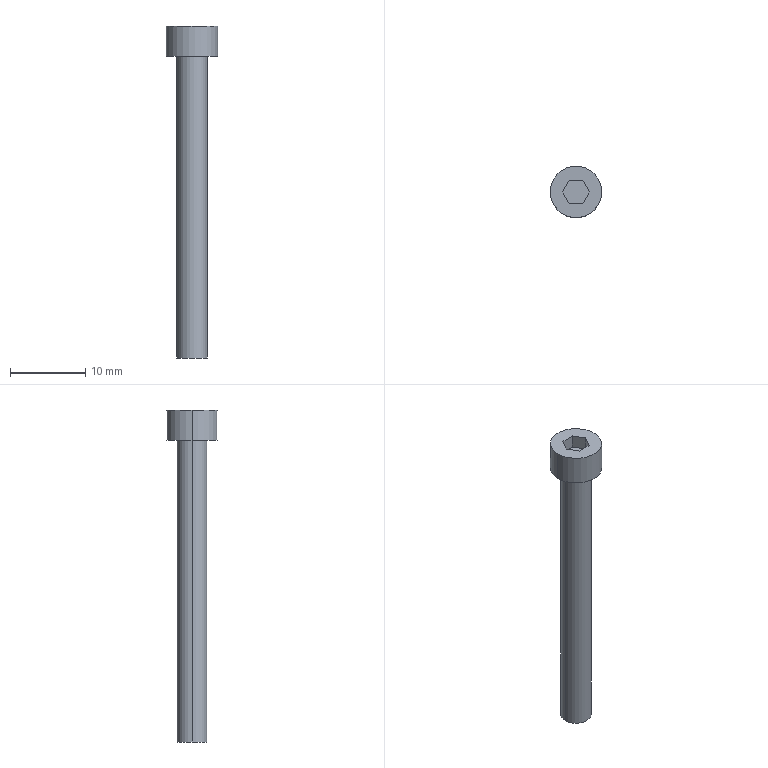Part | SolidWorks | features BaseBody 1 | 1 solid | 14 faces | box 6.8 x 6.8 x 44 mm | volume 632.77 mm3 | plane 10 | cylinder 4 | commonest cylinder face diameters 4 x2 6.8 x2
STEP:
#1=CARTESIAN_POINT('',(2.,0.,-40.));
#2=VERTEX_POINT('',#1);
#3=CARTESIAN_POINT('',(-2.,0.,-40.));
#4=VERTEX_POINT('',#3);
#5=CARTESIAN_POINT('',(0.,0.,-40.));
#6=DIRECTION('',(0.,0.,1.));
#7=DIRECTION('',(1.,0.,0.));
#8=AXIS2_PLACEMENT_3D('',#5,#6,#7);
#9=CIRCLE('',#8,2.);
#10=EDGE_CURVE('',#2,#4,#9,.T.);
#11=ORIENTED_EDGE('',*,*,#10,.T.);
#12=CARTESIAN_POINT('',(-2.,0.,0.));
#13=VERTEX_POINT('',#12);
#14=CARTESIAN_POINT('',(-2.,0.,-40.));
#15=DIRECTION('',(0.,0.,1.));
#16=VECTOR('',#15,1000.);
#17=LINE('',#14,#16);
#18=EDGE_CURVE('',#4,#13,#17,.T.);
#19=ORIENTED_EDGE('',*,*,#18,.T.);
#20=CARTESIAN_POINT('',(2.,0.,0.));
#21=VERTEX_POINT('',#20);
#22=CARTESIAN_POINT('',(0.,0.,0.));
#23=DIRECTION('',(0.,0.,-1.));
#24=DIRECTION('',(1.,0.,0.));
#25=AXIS2_PLACEMENT_3D('',#22,#23,#24);
#26=CIRCLE('',#25,2.);
#27=EDGE_CURVE('',#13,#21,#26,.T.);
#28=ORIENTED_EDGE('',*,*,#27,.T.);
#29=CARTESIAN_POINT('',(2.,0.,-40.));
#30=DIRECTION('',(0.,0.,1.));
#31=VECTOR('',#30,1000.);
#32=LINE('',#29,#31);
#33=EDGE_CURVE('',#2,#21,#32,.T.);
#34=ORIENTED_EDGE('',*,*,#33,.F.);
#35=EDGE_LOOP('',(#11,#19,#28,#34));
#36=FACE_OUTER_BOUND('',#35,.T.);
#37=CARTESIAN_POINT('',(0.,0.,-40.));
#38=DIRECTION('',(0.,0.,1.));
#39=DIRECTION('',(1.,0.,0.));
#40=AXIS2_PLACEMENT_3D('',#37,#38,#39);
#41=CYLINDRICAL_SURFACE('',#40,2.);
#42=ADVANCED_FACE('',(#36),#41,.T.);
#43=CARTESIAN_POINT('',(3.4,0.,0.));
#44=VERTEX_POINT('',#43);
#45=CARTESIAN_POINT('',(-3.4,0.,0.));
#46=VERTEX_POINT('',#45);
#47=CARTESIAN_POINT('',(0.,0.,0.));
#48=DIRECTION('',(0.,0.,1.));
#49=DIRECTION('',(1.,0.,0.));
#50=AXIS2_PLACEMENT_3D('',#47,#48,#49);
#51=CIRCLE('',#50,3.4);
#52=EDGE_CURVE('',#44,#46,#51,.T.);
#53=ORIENTED_EDGE('',*,*,#52,.T.);
#54=CARTESIAN_POINT('',(-3.4,0.,4.));
#55=VERTEX_POINT('',#54);
#56=CARTESIAN_POINT('',(-3.4,0.,0.));
#57=DIRECTION('',(0.,0.,1.));
#58=VECTOR('',#57,1000.);
#59=LINE('',#56,#58);
#60=EDGE_CURVE('',#46,#55,#59,.T.);
#61=ORIENTED_EDGE('',*,*,#60,.T.);
#62=CARTESIAN_POINT('',(3.4,0.,4.));
#63=VERTEX_POINT('',#62);
#64=CARTESIAN_POINT('',(0.,0.,4.));
#65=DIRECTION('',(0.,0.,-1.));
#66=DIRECTION('',(1.,0.,0.));
#67=AXIS2_PLACEMENT_3D('',#64,#65,#66);
#68=CIRCLE('',#67,3.4);
#69=EDGE_CURVE('',#55,#63,#68,.T.);
#70=ORIENTED_EDGE('',*,*,#69,.T.);
#71=CARTESIAN_POINT('',(3.4,0.,0.));
#72=DIRECTION('',(0.,0.,1.));
#73=VECTOR('',#72,1000.);
#74=LINE('',#71,#73);
#75=EDGE_CURVE('',#44,#63,#74,.T.);
#76=ORIENTED_EDGE('',*,*,#75,.F.);
#77=EDGE_LOOP('',(#53,#61,#70,#76));
#78=FACE_OUTER_BOUND('',#77,.T.);
#79=CARTESIAN_POINT('',(0.,0.,0.));
#80=DIRECTION('',(0.,0.,1.));
#81=DIRECTION('',(1.,0.,0.));
#82=AXIS2_PLACEMENT_3D('',#79,#80,#81);
#83=CYLINDRICAL_SURFACE('',#82,3.4);
#84=ADVANCED_FACE('',(#78),#83,.T.);
#85=ORIENTED_EDGE('',*,*,#18,.F.);
#86=CARTESIAN_POINT('',(0.,0.,-40.));
#87=DIRECTION('',(0.,0.,1.));
#88=DIRECTION('',(1.,0.,0.));
#89=AXIS2_PLACEMENT_3D('',#86,#87,#88);
#90=CIRCLE('',#89,2.);
#91=EDGE_CURVE('',#4,#2,#90,.T.);
#92=ORIENTED_EDGE('',*,*,#91,.T.);
#93=ORIENTED_EDGE('',*,*,#33,.T.);
#94=CARTESIAN_POINT('',(0.,0.,0.));
#95=DIRECTION('',(0.,0.,-1.));
#96=DIRECTION('',(1.,0.,0.));
#97=AXIS2_PLACEMENT_3D('',#94,#95,#96);
#98=CIRCLE('',#97,2.);
#99=EDGE_CURVE('',#21,#13,#98,.T.);
#100=ORIENTED_EDGE('',*,*,#99,.T.);
#101=EDGE_LOOP('',(#85,#92,#93,#100));
#102=FACE_OUTER_BOUND('',#101,.T.);
#103=CARTESIAN_POINT('',(0.,0.,-40.));
#104=DIRECTION('',(0.,0.,1.));
#105=DIRECTION('',(1.,0.,0.));
#106=AXIS2_PLACEMENT_3D('',#103,#104,#105);
#107=CYLINDRICAL_SURFACE('',#106,2.);
#108=ADVANCED_FACE('',(#102),#107,.T.);
#109=ORIENTED_EDGE('',*,*,#10,.F.);
#110=ORIENTED_EDGE('',*,*,#91,.F.);
#111=EDGE_LOOP('',(#109,#110));
#112=FACE_OUTER_BOUND('',#111,.T.);
#113=CARTESIAN_POINT('',(0.,0.,-40.));
#114=DIRECTION('',(0.,0.,1.));
#115=DIRECTION('',(1.,0.,0.));
#116=AXIS2_PLACEMENT_3D('',#113,#114,#115);
#117=PLANE('',#116);
#118=ADVANCED_FACE('',(#112),#117,.F.);
#119=ORIENTED_EDGE('',*,*,#99,.F.);
#120=ORIENTED_EDGE('',*,*,#27,.F.);
#121=EDGE_LOOP('',(#119,#120));
#122=FACE_BOUND('',#121,.T.);
#123=ORIENTED_EDGE('',*,*,#52,.F.);
#124=CARTESIAN_POINT('',(0.,0.,0.));
#125=DIRECTION('',(0.,0.,1.));
#126=DIRECTION('',(1.,0.,0.));
#127=AXIS2_PLACEMENT_3D('',#124,#125,#126);
#128=CIRCLE('',#127,3.4);
#129=EDGE_CURVE('',#46,#44,#128,.T.);
#130=ORIENTED_EDGE('',*,*,#129,.F.);
#131=EDGE_LOOP('',(#123,#130));
#132=FACE_OUTER_BOUND('',#131,.T.);
#133=CARTESIAN_POINT('',(0.,0.,0.));
#134=DIRECTION('',(0.,0.,1.));
#135=DIRECTION('',(1.,0.,0.));
#136=AXIS2_PLACEMENT_3D('',#133,#134,#135);
#137=PLANE('',#136);
#138=ADVANCED_FACE('',(#122,#132),#137,.F.);
#139=ORIENTED_EDGE('',*,*,#60,.F.);
#140=ORIENTED_EDGE('',*,*,#129,.T.);
#141=ORIENTED_EDGE('',*,*,#75,.T.);
#142=CARTESIAN_POINT('',(0.,0.,4.));
#143=DIRECTION('',(0.,0.,-1.));
#144=DIRECTION('',(1.,0.,0.));
#145=AXIS2_PLACEMENT_3D('',#142,#143,#144);
#146=CIRCLE('',#145,3.4);
#147=EDGE_CURVE('',#63,#55,#146,.T.);
#148=ORIENTED_EDGE('',*,*,#147,.T.);
#149=EDGE_LOOP('',(#139,#140,#141,#148));
#150=FACE_OUTER_BOUND('',#149,.T.);
#151=CARTESIAN_POINT('',(0.,0.,0.));
#152=DIRECTION('',(0.,0.,1.));
#153=DIRECTION('',(1.,0.,0.));
#154=AXIS2_PLACEMENT_3D('',#151,#152,#153);
#155=CYLINDRICAL_SURFACE('',#154,3.4);
#156=ADVANCED_FACE('',(#150),#155,.T.);
#157=CARTESIAN_POINT('',(-0.9,-1.559,4.));
#158=VERTEX_POINT('',#157);
#159=CARTESIAN_POINT('',(-1.8,0.,4.));
#160=VERTEX_POINT('',#159);
#161=CARTESIAN_POINT('',(-0.9,-1.559,4.));
#162=DIRECTION('',(-0.5,0.866,0.));
#163=VECTOR('',#162,1000.);
#164=LINE('',#161,#163);
#165=EDGE_CURVE('',#158,#160,#164,.T.);
#166=ORIENTED_EDGE('',*,*,#165,.T.);
#167=CARTESIAN_POINT('',(-0.9,1.559,4.));
#168=VERTEX_POINT('',#167);
#169=CARTESIAN_POINT('',(-1.8,0.,4.));
#170=DIRECTION('',(0.5,0.866,0.));
#171=VECTOR('',#170,1000.);
#172=LINE('',#169,#171);
#173=EDGE_CURVE('',#160,#168,#172,.T.);
#174=ORIENTED_EDGE('',*,*,#173,.T.);
#175=CARTESIAN_POINT('',(0.9,1.559,4.));
#176=VERTEX_POINT('',#175);
#177=CARTESIAN_POINT('',(0.,1.559,4.));
#178=DIRECTION('',(1.,0.,0.));
#179=VECTOR('',#178,1000.);
#180=LINE('',#177,#179);
#181=EDGE_CURVE('',#168,#176,#180,.T.);
#182=ORIENTED_EDGE('',*,*,#181,.T.);
#183=CARTESIAN_POINT('',(1.8,0.,4.));
#184=VERTEX_POINT('',#183);
#185=CARTESIAN_POINT('',(0.9,1.559,4.));
#186=DIRECTION('',(0.5,-0.866,0.));
#187=VECTOR('',#186,1000.);
#188=LINE('',#185,#187);
#189=EDGE_CURVE('',#176,#184,#188,.T.);
#190=ORIENTED_EDGE('',*,*,#189,.T.);
#191=CARTESIAN_POINT('',(0.9,-1.559,4.));
#192=VERTEX_POINT('',#191);
#193=CARTESIAN_POINT('',(1.8,0.,4.));
#194=DIRECTION('',(-0.5,-0.866,0.));
#195=VECTOR('',#194,1000.);
#196=LINE('',#193,#195);
#197=EDGE_CURVE('',#184,#192,#196,.T.);
#198=ORIENTED_EDGE('',*,*,#197,.T.);
#199=CARTESIAN_POINT('',(0.,-1.559,4.));
#200=DIRECTION('',(-1.,0.,0.));
#201=VECTOR('',#200,1000.);
#202=LINE('',#199,#201);
#203=EDGE_CURVE('',#192,#158,#202,.T.);
#204=ORIENTED_EDGE('',*,*,#203,.T.);
#205=EDGE_LOOP('',(#166,#174,#182,#190,#198,#204));
#206=FACE_BOUND('',#205,.T.);
#207=ORIENTED_EDGE('',*,*,#147,.F.);
#208=ORIENTED_EDGE('',*,*,#69,.F.);
#209=EDGE_LOOP('',(#207,#208));
#210=FACE_OUTER_BOUND('',#209,.T.);
#211=CARTESIAN_POINT('',(0.,0.,4.));
#212=DIRECTION('',(0.,0.,1.));
#213=DIRECTION('',(1.,0.,0.));
#214=AXIS2_PLACEMENT_3D('',#211,#212,#213);
#215=PLANE('',#214);
#216=ADVANCED_FACE('',(#206,#210),#215,.T.);
#217=ORIENTED_EDGE('',*,*,#173,.F.);
#218=CARTESIAN_POINT('',(-1.8,0.,2.2));
#219=VERTEX_POINT('',#218);
#220=CARTESIAN_POINT('',(-1.8,0.,2.2));
#221=DIRECTION('',(0.,0.,-1.));
#222=VECTOR('',#221,1000.);
#223=LINE('',#220,#222);
#224=EDGE_CURVE('',#160,#219,#223,.T.);
#225=ORIENTED_EDGE('',*,*,#224,.T.);
#226=CARTESIAN_POINT('',(-0.9,1.559,2.2));
#227=VERTEX_POINT('',#226);
#228=CARTESIAN_POINT('',(-0.9,1.559,2.2));
#229=DIRECTION('',(0.5,0.866,0.));
#230=VECTOR('',#229,1000.);
#231=LINE('',#228,#230);
#232=EDGE_CURVE('',#219,#227,#231,.T.);
#233=ORIENTED_EDGE('',*,*,#232,.T.);
#234=CARTESIAN_POINT('',(-0.9,1.559,2.2));
#235=DIRECTION('',(0.,0.,1.));
#236=VECTOR('',#235,1000.);
#237=LINE('',#234,#236);
#238=EDGE_CURVE('',#227,#168,#237,.T.);
#239=ORIENTED_EDGE('',*,*,#238,.T.);
#240=EDGE_LOOP('',(#217,#225,#233,#239));
#241=FACE_OUTER_BOUND('',#240,.T.);
#242=CARTESIAN_POINT('',(-0.9,1.559,2.2));
#243=DIRECTION('',(0.866,-0.5,0.));
#244=DIRECTION('',(0.5,0.866,0.));
#245=AXIS2_PLACEMENT_3D('',#242,#243,#244);
#246=PLANE('',#245);
#247=ADVANCED_FACE('',(#241),#246,.T.);
#248=ORIENTED_EDGE('',*,*,#165,.F.);
#249=CARTESIAN_POINT('',(-0.9,-1.559,2.2));
#250=VERTEX_POINT('',#249);
#251=CARTESIAN_POINT('',(-0.9,-1.559,2.2));
#252=DIRECTION('',(0.,0.,-1.));
#253=VECTOR('',#252,1000.);
#254=LINE('',#251,#253);
#255=EDGE_CURVE('',#158,#250,#254,.T.);
#256=ORIENTED_EDGE('',*,*,#255,.T.);
#257=CARTESIAN_POINT('',(-1.8,0.,2.2));
#258=DIRECTION('',(-0.5,0.866,0.));
#259=VECTOR('',#258,1000.);
#260=LINE('',#257,#259);
#261=EDGE_CURVE('',#250,#219,#260,.T.);
#262=ORIENTED_EDGE('',*,*,#261,.T.);
#263=ORIENTED_EDGE('',*,*,#224,.F.);
#264=EDGE_LOOP('',(#248,#256,#262,#263));
#265=FACE_OUTER_BOUND('',#264,.T.);
#266=CARTESIAN_POINT('',(-1.8,0.,2.2));
#267=DIRECTION('',(0.866,0.5,0.));
#268=DIRECTION('',(-0.5,0.866,0.));
#269=AXIS2_PLACEMENT_3D('',#266,#267,#268);
#270=PLANE('',#269);
#271=ADVANCED_FACE('',(#265),#270,.T.);
#272=ORIENTED_EDGE('',*,*,#203,.F.);
#273=CARTESIAN_POINT('',(0.9,-1.559,2.2));
#274=VERTEX_POINT('',#273);
#275=CARTESIAN_POINT('',(0.9,-1.559,2.2));
#276=DIRECTION('',(0.,0.,-1.));
#277=VECTOR('',#276,1000.);
#278=LINE('',#275,#277);
#279=EDGE_CURVE('',#192,#274,#278,.T.);
#280=ORIENTED_EDGE('',*,*,#279,.T.);
#281=CARTESIAN_POINT('',(-0.9,-1.559,2.2));
#282=DIRECTION('',(-1.,0.,0.));
#283=VECTOR('',#282,1000.);
#284=LINE('',#281,#283);
#285=EDGE_CURVE('',#274,#250,#284,.T.);
#286=ORIENTED_EDGE('',*,*,#285,.T.);
#287=ORIENTED_EDGE('',*,*,#255,.F.);
#288=EDGE_LOOP('',(#272,#280,#286,#287));
#289=FACE_OUTER_BOUND('',#288,.T.);
#290=CARTESIAN_POINT('',(-0.9,-1.559,2.2));
#291=DIRECTION('',(0.,1.,0.));
#292=DIRECTION('',(-1.,0.,0.));
#293=AXIS2_PLACEMENT_3D('',#290,#291,#292);
#294=PLANE('',#293);
#295=ADVANCED_FACE('',(#289),#294,.T.);
#296=ORIENTED_EDGE('',*,*,#197,.F.);
#297=CARTESIAN_POINT('',(1.8,0.,2.2));
#298=VERTEX_POINT('',#297);
#299=CARTESIAN_POINT('',(1.8,0.,2.2));
#300=DIRECTION('',(0.,0.,-1.));
#301=VECTOR('',#300,1000.);
#302=LINE('',#299,#301);
#303=EDGE_CURVE('',#184,#298,#302,.T.);
#304=ORIENTED_EDGE('',*,*,#303,.T.);
#305=CARTESIAN_POINT('',(0.9,-1.559,2.2));
#306=DIRECTION('',(-0.5,-0.866,0.));
#307=VECTOR('',#306,1000.);
#308=LINE('',#305,#307);
#309=EDGE_CURVE('',#298,#274,#308,.T.);
#310=ORIENTED_EDGE('',*,*,#309,.T.);
#311=ORIENTED_EDGE('',*,*,#279,.F.);
#312=EDGE_LOOP('',(#296,#304,#310,#311));
#313=FACE_OUTER_BOUND('',#312,.T.);
#314=CARTESIAN_POINT('',(0.9,-1.559,2.2));
#315=DIRECTION('',(-0.866,0.5,0.));
#316=DIRECTION('',(-0.5,-0.866,0.));
#317=AXIS2_PLACEMENT_3D('',#314,#315,#316);
#318=PLANE('',#317);
#319=ADVANCED_FACE('',(#313),#318,.T.);
#320=ORIENTED_EDGE('',*,*,#189,.F.);
#321=CARTESIAN_POINT('',(0.9,1.559,2.2));
#322=VERTEX_POINT('',#321);
#323=CARTESIAN_POINT('',(0.9,1.559,2.2));
#324=DIRECTION('',(0.,0.,-1.));
#325=VECTOR('',#324,1000.);
#326=LINE('',#323,#325);
#327=EDGE_CURVE('',#176,#322,#326,.T.);
#328=ORIENTED_EDGE('',*,*,#327,.T.);
#329=CARTESIAN_POINT('',(1.8,0.,2.2));
#330=DIRECTION('',(0.5,-0.866,0.));
#331=VECTOR('',#330,1000.);
#332=LINE('',#329,#331);
#333=EDGE_CURVE('',#322,#298,#332,.T.);
#334=ORIENTED_EDGE('',*,*,#333,.T.);
#335=ORIENTED_EDGE('',*,*,#303,.F.);
#336=EDGE_LOOP('',(#320,#328,#334,#335));
#337=FACE_OUTER_BOUND('',#336,.T.);
#338=CARTESIAN_POINT('',(1.8,0.,2.2));
#339=DIRECTION('',(-0.866,-0.5,0.));
#340=DIRECTION('',(0.5,-0.866,0.));
#341=AXIS2_PLACEMENT_3D('',#338,#339,#340);
#342=PLANE('',#341);
#343=ADVANCED_FACE('',(#337),#342,.T.);
#344=ORIENTED_EDGE('',*,*,#181,.F.);
#345=ORIENTED_EDGE('',*,*,#238,.F.);
#346=CARTESIAN_POINT('',(0.9,1.559,2.2));
#347=DIRECTION('',(1.,0.,0.));
#348=VECTOR('',#347,1000.);
#349=LINE('',#346,#348);
#350=EDGE_CURVE('',#227,#322,#349,.T.);
#351=ORIENTED_EDGE('',*,*,#350,.T.);
#352=ORIENTED_EDGE('',*,*,#327,.F.);
#353=EDGE_LOOP('',(#344,#345,#351,#352));
#354=FACE_OUTER_BOUND('',#353,.T.);
#355=CARTESIAN_POINT('',(0.9,1.559,2.2));
#356=DIRECTION('',(0.,-1.,0.));
#357=DIRECTION('',(1.,0.,0.));
#358=AXIS2_PLACEMENT_3D('',#355,#356,#357);
#359=PLANE('',#358);
#360=ADVANCED_FACE('',(#354),#359,.T.);
#361=ORIENTED_EDGE('',*,*,#285,.F.);
#362=ORIENTED_EDGE('',*,*,#309,.F.);
#363=ORIENTED_EDGE('',*,*,#333,.F.);
#364=ORIENTED_EDGE('',*,*,#350,.F.);
#365=ORIENTED_EDGE('',*,*,#232,.F.);
#366=ORIENTED_EDGE('',*,*,#261,.F.);
#367=EDGE_LOOP('',(#361,#362,#363,#364,#365,#366));
#368=FACE_OUTER_BOUND('',#367,.T.);
#369=CARTESIAN_POINT('',(0.,0.,2.2));
#370=DIRECTION('',(0.,0.,1.));
#371=DIRECTION('',(1.,0.,0.));
#372=AXIS2_PLACEMENT_3D('',#369,#370,#371);
#373=PLANE('',#372);
#374=ADVANCED_FACE('',(#368),#373,.T.);
#375=CLOSED_SHELL('',(#42,#84,#108,#118,#138,#156,#216,#247,#271,#295,#319,#343,#360,#374));
#376=MANIFOLD_SOLID_BREP('',#375);
#377=CARTESIAN_POINT('',(0.,0.,0.));
#378=DIRECTION('',(0.,0.,1.));
#379=DIRECTION('',(1.,0.,0.));
#380=AXIS2_PLACEMENT_3D('',#377,#378,#379);
#381=(LENGTH_UNIT()NAMED_UNIT(*)SI_UNIT(.MILLI.,.METRE.));
#382=UNCERTAINTY_MEASURE_WITH_UNIT(LENGTH_MEASURE(0.00001),#381,'','');
#383=(NAMED_UNIT(*)PLANE_ANGLE_UNIT()SI_UNIT($,.RADIAN.));
#384=(NAMED_UNIT(*)SI_UNIT($,.STERADIAN.)SOLID_ANGLE_UNIT());
#385=(GEOMETRIC_REPRESENTATION_CONTEXT(3)GLOBAL_UNCERTAINTY_ASSIGNED_CONTEXT((#382))GLOBAL_UNIT_ASSIGNED_CONTEXT((#381,#383,#384))REPRESENTATION_CONTEXT('',''));
#386=ADVANCED_BREP_SHAPE_REPRESENTATION('',(#376,#380),#385);